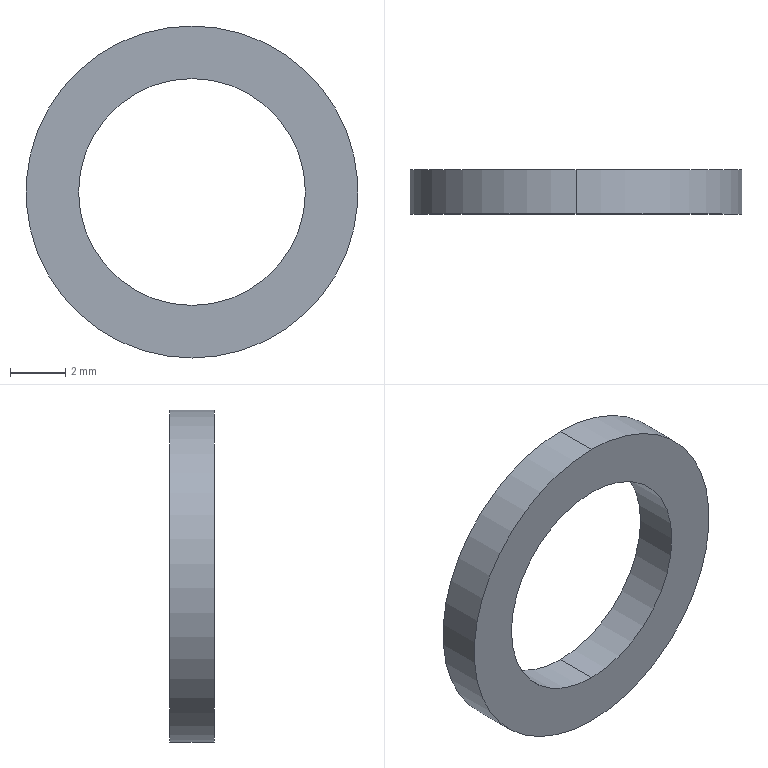Part | SolidWorks | features Extrusion 1 | 1 solid | 6 faces | box 12 x 1.6 x 12 mm | volume 96.459 mm3 | cylinder 4 | plane 2 | commonest cylinder face diameters 8.2 x2 12 x2
STEP:
#1=CARTESIAN_POINT('',(0.,1.6,-4.1));
#2=VERTEX_POINT('',#1);
#3=CARTESIAN_POINT('',(0.,1.6,4.1));
#4=VERTEX_POINT('',#3);
#5=CARTESIAN_POINT('',(0.,1.6,0.));
#6=DIRECTION('',(0.,1.,0.));
#7=DIRECTION('',(0.,0.,1.));
#8=AXIS2_PLACEMENT_3D('',#5,#6,#7);
#9=CIRCLE('',#8,4.1);
#10=EDGE_CURVE('',#2,#4,#9,.T.);
#11=ORIENTED_EDGE('',*,*,#10,.T.);
#12=CARTESIAN_POINT('',(0.,0.,4.1));
#13=VERTEX_POINT('',#12);
#14=CARTESIAN_POINT('',(0.,1.6,4.1));
#15=DIRECTION('',(0.,-1.,0.));
#16=VECTOR('',#15,1000.);
#17=LINE('',#14,#16);
#18=EDGE_CURVE('',#4,#13,#17,.T.);
#19=ORIENTED_EDGE('',*,*,#18,.T.);
#20=CARTESIAN_POINT('',(0.,0.,-4.1));
#21=VERTEX_POINT('',#20);
#22=CARTESIAN_POINT('',(0.,0.,0.));
#23=DIRECTION('',(0.,1.,0.));
#24=DIRECTION('',(0.,0.,1.));
#25=AXIS2_PLACEMENT_3D('',#22,#23,#24);
#26=CIRCLE('',#25,4.1);
#27=EDGE_CURVE('',#21,#13,#26,.T.);
#28=ORIENTED_EDGE('',*,*,#27,.F.);
#29=CARTESIAN_POINT('',(0.,1.6,-4.1));
#30=DIRECTION('',(0.,-1.,0.));
#31=VECTOR('',#30,1000.);
#32=LINE('',#29,#31);
#33=EDGE_CURVE('',#2,#21,#32,.T.);
#34=ORIENTED_EDGE('',*,*,#33,.F.);
#35=EDGE_LOOP('',(#11,#19,#28,#34));
#36=FACE_OUTER_BOUND('',#35,.T.);
#37=CARTESIAN_POINT('',(0.,1.6,0.));
#38=DIRECTION('',(0.,-1.,0.));
#39=DIRECTION('',(0.,0.,-1.));
#40=AXIS2_PLACEMENT_3D('',#37,#38,#39);
#41=CYLINDRICAL_SURFACE('',#40,4.1);
#42=ADVANCED_FACE('',(#36),#41,.F.);
#43=CARTESIAN_POINT('',(0.,1.6,6.));
#44=VERTEX_POINT('',#43);
#45=CARTESIAN_POINT('',(0.,1.6,-6.));
#46=VERTEX_POINT('',#45);
#47=CARTESIAN_POINT('',(0.,1.6,0.));
#48=DIRECTION('',(0.,1.,0.));
#49=DIRECTION('',(0.,0.,1.));
#50=AXIS2_PLACEMENT_3D('',#47,#48,#49);
#51=CIRCLE('',#50,6.);
#52=EDGE_CURVE('',#44,#46,#51,.T.);
#53=ORIENTED_EDGE('',*,*,#52,.F.);
#54=CARTESIAN_POINT('',(0.,0.,6.));
#55=VERTEX_POINT('',#54);
#56=CARTESIAN_POINT('',(0.,1.6,6.));
#57=DIRECTION('',(0.,-1.,0.));
#58=VECTOR('',#57,1000.);
#59=LINE('',#56,#58);
#60=EDGE_CURVE('',#44,#55,#59,.T.);
#61=ORIENTED_EDGE('',*,*,#60,.T.);
#62=CARTESIAN_POINT('',(0.,0.,-6.));
#63=VERTEX_POINT('',#62);
#64=CARTESIAN_POINT('',(0.,0.,0.));
#65=DIRECTION('',(0.,1.,0.));
#66=DIRECTION('',(0.,0.,1.));
#67=AXIS2_PLACEMENT_3D('',#64,#65,#66);
#68=CIRCLE('',#67,6.);
#69=EDGE_CURVE('',#55,#63,#68,.T.);
#70=ORIENTED_EDGE('',*,*,#69,.T.);
#71=CARTESIAN_POINT('',(0.,1.6,-6.));
#72=DIRECTION('',(0.,-1.,0.));
#73=VECTOR('',#72,1000.);
#74=LINE('',#71,#73);
#75=EDGE_CURVE('',#46,#63,#74,.T.);
#76=ORIENTED_EDGE('',*,*,#75,.F.);
#77=EDGE_LOOP('',(#53,#61,#70,#76));
#78=FACE_OUTER_BOUND('',#77,.T.);
#79=CARTESIAN_POINT('',(0.,1.6,0.));
#80=DIRECTION('',(0.,-1.,0.));
#81=DIRECTION('',(0.,0.,-1.));
#82=AXIS2_PLACEMENT_3D('',#79,#80,#81);
#83=CYLINDRICAL_SURFACE('',#82,6.);
#84=ADVANCED_FACE('',(#78),#83,.T.);
#85=CARTESIAN_POINT('',(0.,1.6,0.));
#86=DIRECTION('',(0.,1.,0.));
#87=DIRECTION('',(0.,0.,1.));
#88=AXIS2_PLACEMENT_3D('',#85,#86,#87);
#89=CIRCLE('',#88,6.);
#90=EDGE_CURVE('',#46,#44,#89,.T.);
#91=ORIENTED_EDGE('',*,*,#90,.T.);
#92=ORIENTED_EDGE('',*,*,#52,.T.);
#93=EDGE_LOOP('',(#91,#92));
#94=FACE_OUTER_BOUND('',#93,.T.);
#95=ORIENTED_EDGE('',*,*,#10,.F.);
#96=CARTESIAN_POINT('',(0.,1.6,0.));
#97=DIRECTION('',(0.,1.,0.));
#98=DIRECTION('',(0.,0.,1.));
#99=AXIS2_PLACEMENT_3D('',#96,#97,#98);
#100=CIRCLE('',#99,4.1);
#101=EDGE_CURVE('',#4,#2,#100,.T.);
#102=ORIENTED_EDGE('',*,*,#101,.F.);
#103=EDGE_LOOP('',(#95,#102));
#104=FACE_BOUND('',#103,.T.);
#105=CARTESIAN_POINT('',(0.,1.6,0.));
#106=DIRECTION('',(0.,1.,0.));
#107=DIRECTION('',(0.,0.,1.));
#108=AXIS2_PLACEMENT_3D('',#105,#106,#107);
#109=PLANE('',#108);
#110=ADVANCED_FACE('',(#94,#104),#109,.T.);
#111=CARTESIAN_POINT('',(0.,0.,0.));
#112=DIRECTION('',(0.,1.,0.));
#113=DIRECTION('',(0.,0.,1.));
#114=AXIS2_PLACEMENT_3D('',#111,#112,#113);
#115=CIRCLE('',#114,6.);
#116=EDGE_CURVE('',#63,#55,#115,.T.);
#117=ORIENTED_EDGE('',*,*,#116,.F.);
#118=ORIENTED_EDGE('',*,*,#69,.F.);
#119=EDGE_LOOP('',(#117,#118));
#120=FACE_OUTER_BOUND('',#119,.T.);
#121=ORIENTED_EDGE('',*,*,#27,.T.);
#122=CARTESIAN_POINT('',(0.,0.,0.));
#123=DIRECTION('',(0.,1.,0.));
#124=DIRECTION('',(0.,0.,1.));
#125=AXIS2_PLACEMENT_3D('',#122,#123,#124);
#126=CIRCLE('',#125,4.1);
#127=EDGE_CURVE('',#13,#21,#126,.T.);
#128=ORIENTED_EDGE('',*,*,#127,.T.);
#129=EDGE_LOOP('',(#121,#128));
#130=FACE_BOUND('',#129,.T.);
#131=CARTESIAN_POINT('',(0.,0.,0.));
#132=DIRECTION('',(0.,1.,0.));
#133=DIRECTION('',(0.,0.,1.));
#134=AXIS2_PLACEMENT_3D('',#131,#132,#133);
#135=PLANE('',#134);
#136=ADVANCED_FACE('',(#120,#130),#135,.F.);
#137=ORIENTED_EDGE('',*,*,#60,.F.);
#138=ORIENTED_EDGE('',*,*,#90,.F.);
#139=ORIENTED_EDGE('',*,*,#75,.T.);
#140=ORIENTED_EDGE('',*,*,#116,.T.);
#141=EDGE_LOOP('',(#137,#138,#139,#140));
#142=FACE_OUTER_BOUND('',#141,.T.);
#143=CARTESIAN_POINT('',(0.,1.6,0.));
#144=DIRECTION('',(0.,-1.,0.));
#145=DIRECTION('',(0.,0.,-1.));
#146=AXIS2_PLACEMENT_3D('',#143,#144,#145);
#147=CYLINDRICAL_SURFACE('',#146,6.);
#148=ADVANCED_FACE('',(#142),#147,.T.);
#149=ORIENTED_EDGE('',*,*,#18,.F.);
#150=ORIENTED_EDGE('',*,*,#101,.T.);
#151=ORIENTED_EDGE('',*,*,#33,.T.);
#152=ORIENTED_EDGE('',*,*,#127,.F.);
#153=EDGE_LOOP('',(#149,#150,#151,#152));
#154=FACE_OUTER_BOUND('',#153,.T.);
#155=CARTESIAN_POINT('',(0.,1.6,0.));
#156=DIRECTION('',(0.,-1.,0.));
#157=DIRECTION('',(0.,0.,-1.));
#158=AXIS2_PLACEMENT_3D('',#155,#156,#157);
#159=CYLINDRICAL_SURFACE('',#158,4.1);
#160=ADVANCED_FACE('',(#154),#159,.F.);
#161=CLOSED_SHELL('',(#42,#84,#110,#136,#148,#160));
#162=MANIFOLD_SOLID_BREP('',#161);
#163=CARTESIAN_POINT('',(0.,0.,0.));
#164=DIRECTION('',(0.,0.,1.));
#165=DIRECTION('',(1.,0.,0.));
#166=AXIS2_PLACEMENT_3D('',#163,#164,#165);
#167=(LENGTH_UNIT()NAMED_UNIT(*)SI_UNIT(.MILLI.,.METRE.));
#168=UNCERTAINTY_MEASURE_WITH_UNIT(LENGTH_MEASURE(0.00001),#167,'','');
#169=(NAMED_UNIT(*)PLANE_ANGLE_UNIT()SI_UNIT($,.RADIAN.));
#170=(NAMED_UNIT(*)SI_UNIT($,.STERADIAN.)SOLID_ANGLE_UNIT());
#171=(GEOMETRIC_REPRESENTATION_CONTEXT(3)GLOBAL_UNCERTAINTY_ASSIGNED_CONTEXT((#168))GLOBAL_UNIT_ASSIGNED_CONTEXT((#167,#169,#170))REPRESENTATION_CONTEXT('',''));
#172=ADVANCED_BREP_SHAPE_REPRESENTATION('',(#162,#166),#171);